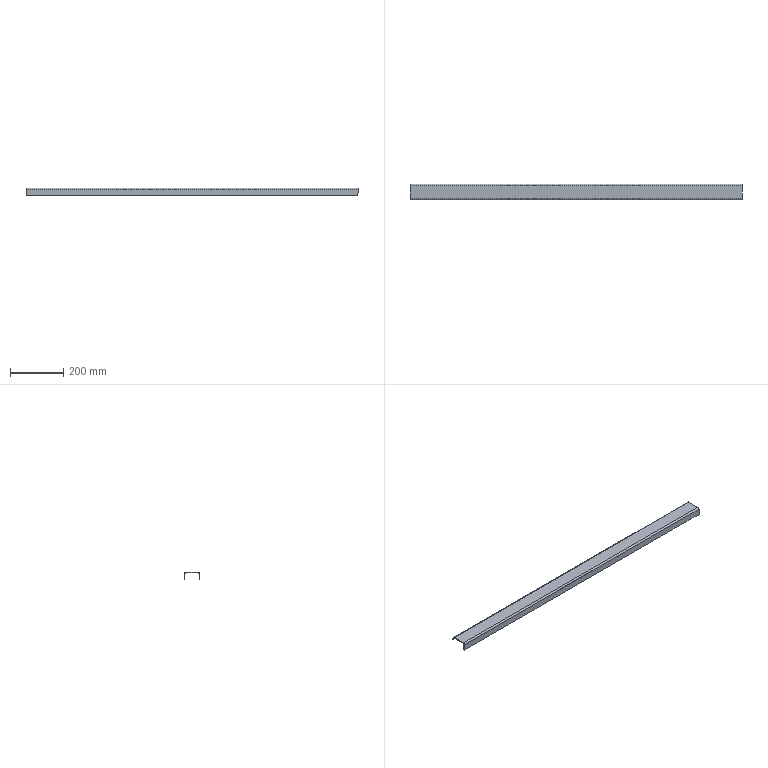Part | SolidWorks | features EdgeFlange 1, Fillet 1, FlatPattern 1, ICE 1, SMBaseFlange 1, SheetMetal 1 | 1 solid | 46 faces | box 1250 x 60 x 30 mm | volume 350614 mm3 | plane 30 | cylinder 16 | commonest cylinder face diameters 12 x14 6 x2
STEP:
#1=CARTESIAN_POINT('',(-29.,30.,-30.));
#2=VERTEX_POINT('',#1);
#3=CARTESIAN_POINT('',(29.,30.,-30.));
#4=VERTEX_POINT('',#3);
#5=CARTESIAN_POINT('',(625.,30.,-30.));
#6=DIRECTION('',(1.,0.,0.));
#7=VECTOR('',#6,1000.);
#8=LINE('',#5,#7);
#9=EDGE_CURVE('',#2,#4,#8,.T.);
#10=ORIENTED_EDGE('',*,*,#9,.T.);
#11=CARTESIAN_POINT('',(29.,27.,-30.));
#12=VERTEX_POINT('',#11);
#13=CARTESIAN_POINT('',(29.,27.,-30.));
#14=DIRECTION('',(0.,-1.,0.));
#15=VECTOR('',#14,1000.);
#16=LINE('',#13,#15);
#17=EDGE_CURVE('',#4,#12,#16,.T.);
#18=ORIENTED_EDGE('',*,*,#17,.T.);
#19=CARTESIAN_POINT('',(-29.,27.,-30.));
#20=VERTEX_POINT('',#19);
#21=CARTESIAN_POINT('',(0.,27.,-30.));
#22=DIRECTION('',(1.,0.,0.));
#23=VECTOR('',#22,1000.);
#24=LINE('',#21,#23);
#25=EDGE_CURVE('',#20,#12,#24,.T.);
#26=ORIENTED_EDGE('',*,*,#25,.F.);
#27=CARTESIAN_POINT('',(-29.,30.,-30.));
#28=DIRECTION('',(0.,1.,0.));
#29=VECTOR('',#28,1000.);
#30=LINE('',#27,#29);
#31=EDGE_CURVE('',#20,#2,#30,.T.);
#32=ORIENTED_EDGE('',*,*,#31,.T.);
#33=EDGE_LOOP('',(#10,#18,#26,#32));
#34=FACE_OUTER_BOUND('',#33,.T.);
#35=CARTESIAN_POINT('',(625.,30.,-30.));
#36=DIRECTION('',(0.,0.,-1.));
#37=DIRECTION('',(0.,1.,0.));
#38=AXIS2_PLACEMENT_3D('',#35,#36,#37);
#39=PLANE('',#38);
#40=ADVANCED_FACE('',(#34),#39,.T.);
#41=CARTESIAN_POINT('',(406.,27.,-30.));
#42=VERTEX_POINT('',#41);
#43=CARTESIAN_POINT('',(464.,27.,-30.));
#44=VERTEX_POINT('',#43);
#45=CARTESIAN_POINT('',(0.,27.,-30.));
#46=DIRECTION('',(1.,0.,0.));
#47=VECTOR('',#46,1000.);
#48=LINE('',#45,#47);
#49=EDGE_CURVE('',#42,#44,#48,.T.);
#50=ORIENTED_EDGE('',*,*,#49,.F.);
#51=CARTESIAN_POINT('',(406.,30.,-30.));
#52=VERTEX_POINT('',#51);
#53=CARTESIAN_POINT('',(406.,30.,-30.));
#54=DIRECTION('',(0.,1.,0.));
#55=VECTOR('',#54,1000.);
#56=LINE('',#53,#55);
#57=EDGE_CURVE('',#42,#52,#56,.T.);
#58=ORIENTED_EDGE('',*,*,#57,.T.);
#59=CARTESIAN_POINT('',(464.,30.,-30.));
#60=VERTEX_POINT('',#59);
#61=CARTESIAN_POINT('',(625.,30.,-30.));
#62=DIRECTION('',(1.,0.,0.));
#63=VECTOR('',#62,1000.);
#64=LINE('',#61,#63);
#65=EDGE_CURVE('',#52,#60,#64,.T.);
#66=ORIENTED_EDGE('',*,*,#65,.T.);
#67=CARTESIAN_POINT('',(464.,27.,-30.));
#68=DIRECTION('',(0.,-1.,0.));
#69=VECTOR('',#68,1000.);
#70=LINE('',#67,#69);
#71=EDGE_CURVE('',#60,#44,#70,.T.);
#72=ORIENTED_EDGE('',*,*,#71,.T.);
#73=EDGE_LOOP('',(#50,#58,#66,#72));
#74=FACE_OUTER_BOUND('',#73,.T.);
#75=CARTESIAN_POINT('',(625.,30.,-30.));
#76=DIRECTION('',(0.,0.,-1.));
#77=DIRECTION('',(0.,1.,0.));
#78=AXIS2_PLACEMENT_3D('',#75,#76,#77);
#79=PLANE('',#78);
#80=ADVANCED_FACE('',(#74),#79,.T.);
#81=CARTESIAN_POINT('',(625.,-24.,-3.));
#82=VERTEX_POINT('',#81);
#83=CARTESIAN_POINT('',(625.,24.,-3.));
#84=VERTEX_POINT('',#83);
#85=CARTESIAN_POINT('',(625.,-30.,-3.));
#86=DIRECTION('',(0.,1.,0.));
#87=VECTOR('',#86,1000.);
#88=LINE('',#85,#87);
#89=EDGE_CURVE('',#82,#84,#88,.T.);
#90=ORIENTED_EDGE('',*,*,#89,.F.);
#91=CARTESIAN_POINT('',(-625.,-24.,-3.));
#92=VERTEX_POINT('',#91);
#93=CARTESIAN_POINT('',(-625.,-24.,-3.));
#94=DIRECTION('',(1.,0.,0.));
#95=VECTOR('',#94,1000.);
#96=LINE('',#93,#95);
#97=EDGE_CURVE('',#92,#82,#96,.T.);
#98=ORIENTED_EDGE('',*,*,#97,.F.);
#99=CARTESIAN_POINT('',(-625.,24.,-3.));
#100=VERTEX_POINT('',#99);
#101=CARTESIAN_POINT('',(-625.,-30.,-3.));
#102=DIRECTION('',(0.,-1.,0.));
#103=VECTOR('',#102,1000.);
#104=LINE('',#101,#103);
#105=EDGE_CURVE('',#100,#92,#104,.T.);
#106=ORIENTED_EDGE('',*,*,#105,.F.);
#107=CARTESIAN_POINT('',(625.,24.,-3.));
#108=DIRECTION('',(-1.,0.,0.));
#109=VECTOR('',#108,1000.);
#110=LINE('',#107,#109);
#111=EDGE_CURVE('',#84,#100,#110,.T.);
#112=ORIENTED_EDGE('',*,*,#111,.F.);
#113=EDGE_LOOP('',(#90,#98,#106,#112));
#114=FACE_OUTER_BOUND('',#113,.T.);
#115=CARTESIAN_POINT('',(0.,0.,-3.));
#116=DIRECTION('',(0.,0.,-1.));
#117=DIRECTION('',(-1.,0.,0.));
#118=AXIS2_PLACEMENT_3D('',#115,#116,#117);
#119=PLANE('',#118);
#120=ADVANCED_FACE('',(#114),#119,.T.);
#121=CARTESIAN_POINT('',(-625.,-24.,0.));
#122=VERTEX_POINT('',#121);
#123=CARTESIAN_POINT('',(625.,-24.,0.));
#124=VERTEX_POINT('',#123);
#125=CARTESIAN_POINT('',(-625.,-24.,0.));
#126=DIRECTION('',(1.,0.,0.));
#127=VECTOR('',#126,1000.);
#128=LINE('',#125,#127);
#129=EDGE_CURVE('',#122,#124,#128,.T.);
#130=ORIENTED_EDGE('',*,*,#129,.T.);
#131=CARTESIAN_POINT('',(625.,24.,0.));
#132=VERTEX_POINT('',#131);
#133=CARTESIAN_POINT('',(625.,-30.,0.));
#134=DIRECTION('',(0.,1.,0.));
#135=VECTOR('',#134,1000.);
#136=LINE('',#133,#135);
#137=EDGE_CURVE('',#124,#132,#136,.T.);
#138=ORIENTED_EDGE('',*,*,#137,.T.);
#139=CARTESIAN_POINT('',(-625.,24.,0.));
#140=VERTEX_POINT('',#139);
#141=CARTESIAN_POINT('',(625.,24.,0.));
#142=DIRECTION('',(-1.,0.,0.));
#143=VECTOR('',#142,1000.);
#144=LINE('',#141,#143);
#145=EDGE_CURVE('',#132,#140,#144,.T.);
#146=ORIENTED_EDGE('',*,*,#145,.T.);
#147=CARTESIAN_POINT('',(-625.,-30.,0.));
#148=DIRECTION('',(0.,-1.,0.));
#149=VECTOR('',#148,1000.);
#150=LINE('',#147,#149);
#151=EDGE_CURVE('',#140,#122,#150,.T.);
#152=ORIENTED_EDGE('',*,*,#151,.T.);
#153=EDGE_LOOP('',(#130,#138,#146,#152));
#154=FACE_OUTER_BOUND('',#153,.T.);
#155=CARTESIAN_POINT('',(0.,0.,0.));
#156=DIRECTION('',(0.,0.,-1.));
#157=DIRECTION('',(-1.,0.,0.));
#158=AXIS2_PLACEMENT_3D('',#155,#156,#157);
#159=PLANE('',#158);
#160=ADVANCED_FACE('',(#154),#159,.F.);
#161=ORIENTED_EDGE('',*,*,#105,.T.);
#162=CARTESIAN_POINT('',(-625.,-24.,-3.));
#163=DIRECTION('',(0.,0.,1.));
#164=VECTOR('',#163,1000.);
#165=LINE('',#162,#164);
#166=EDGE_CURVE('',#92,#122,#165,.T.);
#167=ORIENTED_EDGE('',*,*,#166,.T.);
#168=ORIENTED_EDGE('',*,*,#151,.F.);
#169=CARTESIAN_POINT('',(-625.,24.,-3.));
#170=DIRECTION('',(0.,0.,1.));
#171=VECTOR('',#170,1000.);
#172=LINE('',#169,#171);
#173=EDGE_CURVE('',#100,#140,#172,.T.);
#174=ORIENTED_EDGE('',*,*,#173,.F.);
#175=EDGE_LOOP('',(#161,#167,#168,#174));
#176=FACE_OUTER_BOUND('',#175,.T.);
#177=CARTESIAN_POINT('',(-625.,-30.,-3.));
#178=DIRECTION('',(-1.,0.,0.));
#179=DIRECTION('',(0.,0.,1.));
#180=AXIS2_PLACEMENT_3D('',#177,#178,#179);
#181=PLANE('',#180);
#182=ADVANCED_FACE('',(#176),#181,.T.);
#183=CARTESIAN_POINT('',(625.,-24.,-3.));
#184=DIRECTION('',(0.,0.,1.));
#185=VECTOR('',#184,1000.);
#186=LINE('',#183,#185);
#187=EDGE_CURVE('',#82,#124,#186,.T.);
#188=ORIENTED_EDGE('',*,*,#187,.F.);
#189=ORIENTED_EDGE('',*,*,#89,.T.);
#190=CARTESIAN_POINT('',(625.,24.,-3.));
#191=DIRECTION('',(0.,0.,1.));
#192=VECTOR('',#191,1000.);
#193=LINE('',#190,#192);
#194=EDGE_CURVE('',#84,#132,#193,.T.);
#195=ORIENTED_EDGE('',*,*,#194,.T.);
#196=ORIENTED_EDGE('',*,*,#137,.F.);
#197=EDGE_LOOP('',(#188,#189,#195,#196));
#198=FACE_OUTER_BOUND('',#197,.T.);
#199=CARTESIAN_POINT('',(625.,-30.,-3.));
#200=DIRECTION('',(1.,0.,0.));
#201=DIRECTION('',(0.,0.,-1.));
#202=AXIS2_PLACEMENT_3D('',#199,#200,#201);
#203=PLANE('',#202);
#204=ADVANCED_FACE('',(#198),#203,.T.);
#205=CARTESIAN_POINT('',(-625.,27.,-6.));
#206=VERTEX_POINT('',#205);
#207=CARTESIAN_POINT('',(-625.,30.,-6.));
#208=VERTEX_POINT('',#207);
#209=CARTESIAN_POINT('',(-625.,30.,-6.));
#210=DIRECTION('',(0.,1.,0.));
#211=VECTOR('',#210,1000.);
#212=LINE('',#209,#211);
#213=EDGE_CURVE('',#206,#208,#212,.T.);
#214=ORIENTED_EDGE('',*,*,#213,.F.);
#215=CARTESIAN_POINT('',(-625.,24.,-6.));
#216=DIRECTION('',(-1.,0.,0.));
#217=DIRECTION('',(0.,0.,-1.));
#218=AXIS2_PLACEMENT_3D('',#215,#216,#217);
#219=CIRCLE('',#218,3.);
#220=EDGE_CURVE('',#100,#206,#219,.T.);
#221=ORIENTED_EDGE('',*,*,#220,.F.);
#222=ORIENTED_EDGE('',*,*,#173,.T.);
#223=CARTESIAN_POINT('',(-625.,24.,-6.));
#224=DIRECTION('',(-1.,0.,0.));
#225=DIRECTION('',(0.,0.,-1.));
#226=AXIS2_PLACEMENT_3D('',#223,#224,#225);
#227=CIRCLE('',#226,6.);
#228=EDGE_CURVE('',#140,#208,#227,.T.);
#229=ORIENTED_EDGE('',*,*,#228,.T.);
#230=EDGE_LOOP('',(#214,#221,#222,#229));
#231=FACE_OUTER_BOUND('',#230,.T.);
#232=CARTESIAN_POINT('',(-625.,24.,-6.));
#233=DIRECTION('',(-1.,0.,0.));
#234=DIRECTION('',(0.,0.,1.));
#235=AXIS2_PLACEMENT_3D('',#232,#233,#234);
#236=PLANE('',#235);
#237=ADVANCED_FACE('',(#231),#236,.T.);
#238=CARTESIAN_POINT('',(625.,27.,-6.));
#239=VERTEX_POINT('',#238);
#240=CARTESIAN_POINT('',(625.,24.,-6.));
#241=DIRECTION('',(1.,0.,0.));
#242=DIRECTION('',(0.,0.,-1.));
#243=AXIS2_PLACEMENT_3D('',#240,#241,#242);
#244=CIRCLE('',#243,3.);
#245=EDGE_CURVE('',#239,#84,#244,.T.);
#246=ORIENTED_EDGE('',*,*,#245,.F.);
#247=CARTESIAN_POINT('',(625.,30.,-6.));
#248=VERTEX_POINT('',#247);
#249=CARTESIAN_POINT('',(625.,27.,-6.));
#250=DIRECTION('',(0.,1.,0.));
#251=VECTOR('',#250,1000.);
#252=LINE('',#249,#251);
#253=EDGE_CURVE('',#239,#248,#252,.T.);
#254=ORIENTED_EDGE('',*,*,#253,.T.);
#255=CARTESIAN_POINT('',(625.,24.,-6.));
#256=DIRECTION('',(1.,0.,0.));
#257=DIRECTION('',(0.,0.,-1.));
#258=AXIS2_PLACEMENT_3D('',#255,#256,#257);
#259=CIRCLE('',#258,6.);
#260=EDGE_CURVE('',#248,#132,#259,.T.);
#261=ORIENTED_EDGE('',*,*,#260,.T.);
#262=ORIENTED_EDGE('',*,*,#194,.F.);
#263=EDGE_LOOP('',(#246,#254,#261,#262));
#264=FACE_OUTER_BOUND('',#263,.T.);
#265=CARTESIAN_POINT('',(625.,24.,-6.));
#266=DIRECTION('',(-1.,0.,0.));
#267=DIRECTION('',(0.,0.,1.));
#268=AXIS2_PLACEMENT_3D('',#265,#266,#267);
#269=PLANE('',#268);
#270=ADVANCED_FACE('',(#264),#269,.F.);
#271=ORIENTED_EDGE('',*,*,#145,.F.);
#272=ORIENTED_EDGE('',*,*,#260,.F.);
#273=CARTESIAN_POINT('',(0.,30.,-6.));
#274=DIRECTION('',(1.,0.,0.));
#275=VECTOR('',#274,1000.);
#276=LINE('',#273,#275);
#277=EDGE_CURVE('',#208,#248,#276,.T.);
#278=ORIENTED_EDGE('',*,*,#277,.F.);
#279=ORIENTED_EDGE('',*,*,#228,.F.);
#280=EDGE_LOOP('',(#271,#272,#278,#279));
#281=FACE_OUTER_BOUND('',#280,.T.);
#282=CARTESIAN_POINT('',(625.,24.,-6.));
#283=DIRECTION('',(1.,0.,0.));
#284=DIRECTION('',(0.,1.,0.));
#285=AXIS2_PLACEMENT_3D('',#282,#283,#284);
#286=CYLINDRICAL_SURFACE('',#285,6.);
#287=ADVANCED_FACE('',(#281),#286,.T.);
#288=ORIENTED_EDGE('',*,*,#111,.T.);
#289=ORIENTED_EDGE('',*,*,#220,.T.);
#290=CARTESIAN_POINT('',(-625.,27.,-6.));
#291=DIRECTION('',(1.,0.,0.));
#292=VECTOR('',#291,1000.);
#293=LINE('',#290,#292);
#294=EDGE_CURVE('',#206,#239,#293,.T.);
#295=ORIENTED_EDGE('',*,*,#294,.T.);
#296=ORIENTED_EDGE('',*,*,#245,.T.);
#297=EDGE_LOOP('',(#288,#289,#295,#296));
#298=FACE_OUTER_BOUND('',#297,.T.);
#299=CARTESIAN_POINT('',(625.,24.,-6.));
#300=DIRECTION('',(1.,0.,0.));
#301=DIRECTION('',(0.,1.,0.));
#302=AXIS2_PLACEMENT_3D('',#299,#300,#301);
#303=CYLINDRICAL_SURFACE('',#302,3.);
#304=ADVANCED_FACE('',(#298),#303,.F.);
#305=CARTESIAN_POINT('',(625.,27.,-10.));
#306=VERTEX_POINT('',#305);
#307=CARTESIAN_POINT('',(625.,30.,-10.));
#308=VERTEX_POINT('',#307);
#309=CARTESIAN_POINT('',(625.,20.,-10.));
#310=DIRECTION('',(0.,1.,0.));
#311=VECTOR('',#310,1000.);
#312=LINE('',#309,#311);
#313=EDGE_CURVE('',#306,#308,#312,.T.);
#314=ORIENTED_EDGE('',*,*,#313,.T.);
#315=CARTESIAN_POINT('',(625.,30.,-3.));
#316=DIRECTION('',(0.,0.,1.));
#317=VECTOR('',#316,1000.);
#318=LINE('',#315,#317);
#319=EDGE_CURVE('',#308,#248,#318,.T.);
#320=ORIENTED_EDGE('',*,*,#319,.T.);
#321=ORIENTED_EDGE('',*,*,#253,.F.);
#322=CARTESIAN_POINT('',(625.,27.,0.));
#323=DIRECTION('',(0.,0.,1.));
#324=VECTOR('',#323,1000.);
#325=LINE('',#322,#324);
#326=EDGE_CURVE('',#306,#239,#325,.T.);
#327=ORIENTED_EDGE('',*,*,#326,.F.);
#328=EDGE_LOOP('',(#314,#320,#321,#327));
#329=FACE_OUTER_BOUND('',#328,.T.);
#330=CARTESIAN_POINT('',(625.,30.,-3.));
#331=DIRECTION('',(1.,0.,0.));
#332=DIRECTION('',(0.,0.,-1.));
#333=AXIS2_PLACEMENT_3D('',#330,#331,#332);
#334=PLANE('',#333);
#335=ADVANCED_FACE('',(#329),#334,.T.);
#336=CARTESIAN_POINT('',(-625.,27.,-10.));
#337=VERTEX_POINT('',#336);
#338=CARTESIAN_POINT('',(-625.,30.,-10.));
#339=VERTEX_POINT('',#338);
#340=CARTESIAN_POINT('',(-625.,20.,-10.));
#341=DIRECTION('',(0.,1.,0.));
#342=VECTOR('',#341,1000.);
#343=LINE('',#340,#342);
#344=EDGE_CURVE('',#337,#339,#343,.T.);
#345=ORIENTED_EDGE('',*,*,#344,.F.);
#346=CARTESIAN_POINT('',(-625.,27.,0.));
#347=DIRECTION('',(0.,0.,-1.));
#348=VECTOR('',#347,1000.);
#349=LINE('',#346,#348);
#350=EDGE_CURVE('',#206,#337,#349,.T.);
#351=ORIENTED_EDGE('',*,*,#350,.F.);
#352=ORIENTED_EDGE('',*,*,#213,.T.);
#353=CARTESIAN_POINT('',(-625.,30.,-30.));
#354=DIRECTION('',(0.,0.,-1.));
#355=VECTOR('',#354,1000.);
#356=LINE('',#353,#355);
#357=EDGE_CURVE('',#208,#339,#356,.T.);
#358=ORIENTED_EDGE('',*,*,#357,.T.);
#359=EDGE_LOOP('',(#345,#351,#352,#358));
#360=FACE_OUTER_BOUND('',#359,.T.);
#361=CARTESIAN_POINT('',(-625.,30.,-30.));
#362=DIRECTION('',(-1.,0.,0.));
#363=DIRECTION('',(0.,0.,1.));
#364=AXIS2_PLACEMENT_3D('',#361,#362,#363);
#365=PLANE('',#364);
#366=ADVANCED_FACE('',(#360),#365,.T.);
#367=CARTESIAN_POINT('',(-464.,30.,-30.));
#368=VERTEX_POINT('',#367);
#369=CARTESIAN_POINT('',(-406.,30.,-30.));
#370=VERTEX_POINT('',#369);
#371=CARTESIAN_POINT('',(625.,30.,-30.));
#372=DIRECTION('',(1.,0.,0.));
#373=VECTOR('',#372,1000.);
#374=LINE('',#371,#373);
#375=EDGE_CURVE('',#368,#370,#374,.T.);
#376=ORIENTED_EDGE('',*,*,#375,.F.);
#377=CARTESIAN_POINT('',(-470.,30.,-24.));
#378=VERTEX_POINT('',#377);
#379=CARTESIAN_POINT('',(-464.,30.,-24.));
#380=DIRECTION('',(0.,1.,0.));
#381=DIRECTION('',(0.,0.,1.));
#382=AXIS2_PLACEMENT_3D('',#379,#380,#381);
#383=CIRCLE('',#382,6.);
#384=EDGE_CURVE('',#368,#378,#383,.T.);
#385=ORIENTED_EDGE('',*,*,#384,.T.);
#386=CARTESIAN_POINT('',(-470.,30.,-16.));
#387=VERTEX_POINT('',#386);
#388=CARTESIAN_POINT('',(-470.,30.,-30.));
#389=DIRECTION('',(0.,0.,-1.));
#390=VECTOR('',#389,1000.);
#391=LINE('',#388,#390);
#392=EDGE_CURVE('',#387,#378,#391,.T.);
#393=ORIENTED_EDGE('',*,*,#392,.F.);
#394=CARTESIAN_POINT('',(-476.,30.,-10.));
#395=VERTEX_POINT('',#394);
#396=CARTESIAN_POINT('',(-476.,30.,-16.));
#397=DIRECTION('',(0.,-1.,0.));
#398=DIRECTION('',(0.,0.,1.));
#399=AXIS2_PLACEMENT_3D('',#396,#397,#398);
#400=CIRCLE('',#399,6.);
#401=EDGE_CURVE('',#387,#395,#400,.T.);
#402=ORIENTED_EDGE('',*,*,#401,.T.);
#403=CARTESIAN_POINT('',(-470.,30.,-10.));
#404=DIRECTION('',(1.,0.,0.));
#405=VECTOR('',#404,1000.);
#406=LINE('',#403,#405);
#407=EDGE_CURVE('',#339,#395,#406,.T.);
#408=ORIENTED_EDGE('',*,*,#407,.F.);
#409=ORIENTED_EDGE('',*,*,#357,.F.);
#410=ORIENTED_EDGE('',*,*,#277,.T.);
#411=ORIENTED_EDGE('',*,*,#319,.F.);
#412=CARTESIAN_POINT('',(476.,30.,-10.));
#413=VERTEX_POINT('',#412);
#414=CARTESIAN_POINT('',(470.,30.,-10.));
#415=DIRECTION('',(1.,0.,0.));
#416=VECTOR('',#415,1000.);
#417=LINE('',#414,#416);
#418=EDGE_CURVE('',#413,#308,#417,.T.);
#419=ORIENTED_EDGE('',*,*,#418,.F.);
#420=CARTESIAN_POINT('',(470.,30.,-16.));
#421=VERTEX_POINT('',#420);
#422=CARTESIAN_POINT('',(476.,30.,-16.));
#423=DIRECTION('',(0.,-1.,0.));
#424=DIRECTION('',(0.,0.,1.));
#425=AXIS2_PLACEMENT_3D('',#422,#423,#424);
#426=CIRCLE('',#425,6.);
#427=EDGE_CURVE('',#413,#421,#426,.T.);
#428=ORIENTED_EDGE('',*,*,#427,.T.);
#429=CARTESIAN_POINT('',(470.,30.,-24.));
#430=VERTEX_POINT('',#429);
#431=CARTESIAN_POINT('',(470.,30.,-30.));
#432=DIRECTION('',(0.,0.,1.));
#433=VECTOR('',#432,1000.);
#434=LINE('',#431,#433);
#435=EDGE_CURVE('',#430,#421,#434,.T.);
#436=ORIENTED_EDGE('',*,*,#435,.F.);
#437=CARTESIAN_POINT('',(464.,30.,-24.));
#438=DIRECTION('',(0.,1.,0.));
#439=DIRECTION('',(0.,0.,1.));
#440=AXIS2_PLACEMENT_3D('',#437,#438,#439);
#441=CIRCLE('',#440,6.);
#442=EDGE_CURVE('',#430,#60,#441,.T.);
#443=ORIENTED_EDGE('',*,*,#442,.T.);
#444=ORIENTED_EDGE('',*,*,#65,.F.);
#445=CARTESIAN_POINT('',(400.,30.,-24.));
#446=VERTEX_POINT('',#445);
#447=CARTESIAN_POINT('',(406.,30.,-24.));
#448=DIRECTION('',(0.,1.,0.));
#449=DIRECTION('',(0.,0.,1.));
#450=AXIS2_PLACEMENT_3D('',#447,#448,#449);
#451=CIRCLE('',#450,6.);
#452=EDGE_CURVE('',#52,#446,#451,.T.);
#453=ORIENTED_EDGE('',*,*,#452,.T.);
#454=CARTESIAN_POINT('',(400.,30.,-16.));
#455=VERTEX_POINT('',#454);
#456=CARTESIAN_POINT('',(400.,30.,-30.));
#457=DIRECTION('',(0.,0.,-1.));
#458=VECTOR('',#457,1000.);
#459=LINE('',#456,#458);
#460=EDGE_CURVE('',#455,#446,#459,.T.);
#461=ORIENTED_EDGE('',*,*,#460,.F.);
#462=CARTESIAN_POINT('',(394.,30.,-10.));
#463=VERTEX_POINT('',#462);
#464=CARTESIAN_POINT('',(394.,30.,-16.));
#465=DIRECTION('',(0.,-1.,0.));
#466=DIRECTION('',(0.,0.,1.));
#467=AXIS2_PLACEMENT_3D('',#464,#465,#466);
#468=CIRCLE('',#467,6.);
#469=EDGE_CURVE('',#455,#463,#468,.T.);
#470=ORIENTED_EDGE('',*,*,#469,.T.);
#471=CARTESIAN_POINT('',(41.,30.,-10.));
#472=VERTEX_POINT('',#471);
#473=CARTESIAN_POINT('',(400.,30.,-10.));
#474=DIRECTION('',(1.,0.,0.));
#475=VECTOR('',#474,1000.);
#476=LINE('',#473,#475);
#477=EDGE_CURVE('',#472,#463,#476,.T.);
#478=ORIENTED_EDGE('',*,*,#477,.F.);
#479=CARTESIAN_POINT('',(35.,30.,-16.));
#480=VERTEX_POINT('',#479);
#481=CARTESIAN_POINT('',(41.,30.,-16.));
#482=DIRECTION('',(0.,-1.,0.));
#483=DIRECTION('',(0.,0.,1.));
#484=AXIS2_PLACEMENT_3D('',#481,#482,#483);
#485=CIRCLE('',#484,6.);
#486=EDGE_CURVE('',#472,#480,#485,.T.);
#487=ORIENTED_EDGE('',*,*,#486,.T.);
#488=CARTESIAN_POINT('',(35.,30.,-24.));
#489=VERTEX_POINT('',#488);
#490=CARTESIAN_POINT('',(35.,30.,-30.));
#491=DIRECTION('',(0.,0.,1.));
#492=VECTOR('',#491,1000.);
#493=LINE('',#490,#492);
#494=EDGE_CURVE('',#489,#480,#493,.T.);
#495=ORIENTED_EDGE('',*,*,#494,.F.);
#496=CARTESIAN_POINT('',(29.,30.,-24.));
#497=DIRECTION('',(0.,1.,0.));
#498=DIRECTION('',(0.,0.,1.));
#499=AXIS2_PLACEMENT_3D('',#496,#497,#498);
#500=CIRCLE('',#499,6.);
#501=EDGE_CURVE('',#489,#4,#500,.T.);
#502=ORIENTED_EDGE('',*,*,#501,.T.);
#503=ORIENTED_EDGE('',*,*,#9,.F.);
#504=CARTESIAN_POINT('',(-35.,30.,-24.));
#505=VERTEX_POINT('',#504);
#506=CARTESIAN_POINT('',(-29.,30.,-24.));
#507=DIRECTION('',(0.,1.,0.));
#508=DIRECTION('',(0.,0.,1.));
#509=AXIS2_PLACEMENT_3D('',#506,#507,#508);
#510=CIRCLE('',#509,6.);
#511=EDGE_CURVE('',#2,#505,#510,.T.);
#512=ORIENTED_EDGE('',*,*,#511,.T.);
#513=CARTESIAN_POINT('',(-35.,30.,-16.));
#514=VERTEX_POINT('',#513);
#515=CARTESIAN_POINT('',(-35.,30.,-30.));
#516=DIRECTION('',(0.,0.,-1.));
#517=VECTOR('',#516,1000.);
#518=LINE('',#515,#517);
#519=EDGE_CURVE('',#514,#505,#518,.T.);
#520=ORIENTED_EDGE('',*,*,#519,.F.);
#521=CARTESIAN_POINT('',(-41.,30.,-10.));
#522=VERTEX_POINT('',#521);
#523=CARTESIAN_POINT('',(-41.,30.,-16.));
#524=DIRECTION('',(0.,-1.,0.));
#525=DIRECTION('',(0.,0.,1.));
#526=AXIS2_PLACEMENT_3D('',#523,#524,#525);
#527=CIRCLE('',#526,6.);
#528=EDGE_CURVE('',#514,#522,#527,.T.);
#529=ORIENTED_EDGE('',*,*,#528,.T.);
#530=CARTESIAN_POINT('',(-394.,30.,-10.));
#531=VERTEX_POINT('',#530);
#532=CARTESIAN_POINT('',(-35.,30.,-10.));
#533=DIRECTION('',(1.,0.,0.));
#534=VECTOR('',#533,1000.);
#535=LINE('',#532,#534);
#536=EDGE_CURVE('',#531,#522,#535,.T.);
#537=ORIENTED_EDGE('',*,*,#536,.F.);
#538=CARTESIAN_POINT('',(-400.,30.,-16.));
#539=VERTEX_POINT('',#538);
#540=CARTESIAN_POINT('',(-394.,30.,-16.));
#541=DIRECTION('',(0.,-1.,0.));
#542=DIRECTION('',(0.,0.,1.));
#543=AXIS2_PLACEMENT_3D('',#540,#541,#542);
#544=CIRCLE('',#543,6.);
#545=EDGE_CURVE('',#531,#539,#544,.T.);
#546=ORIENTED_EDGE('',*,*,#545,.T.);
#547=CARTESIAN_POINT('',(-400.,30.,-24.));
#548=VERTEX_POINT('',#547);
#549=CARTESIAN_POINT('',(-400.,30.,-30.));
#550=DIRECTION('',(0.,0.,1.));
#551=VECTOR('',#550,1000.);
#552=LINE('',#549,#551);
#553=EDGE_CURVE('',#548,#539,#552,.T.);
#554=ORIENTED_EDGE('',*,*,#553,.F.);
#555=CARTESIAN_POINT('',(-406.,30.,-24.));
#556=DIRECTION('',(0.,1.,0.));
#557=DIRECTION('',(0.,0.,1.));
#558=AXIS2_PLACEMENT_3D('',#555,#556,#557);
#559=CIRCLE('',#558,6.);
#560=EDGE_CURVE('',#548,#370,#559,.T.);
#561=ORIENTED_EDGE('',*,*,#560,.T.);
#562=EDGE_LOOP('',(#376,#385,#393,#402,#408,#409,#410,#411,#419,#428,#436,#443,#444,#453,#461,#470,#478,#487,#495,#502,#503,#512,#520,#529,#537,#546,#554,#561));
#563=FACE_OUTER_BOUND('',#562,.T.);
#564=CARTESIAN_POINT('',(0.,30.,0.));
#565=DIRECTION('',(0.,1.,0.));
#566=DIRECTION('',(0.,0.,1.));
#567=AXIS2_PLACEMENT_3D('',#564,#565,#566);
#568=PLANE('',#567);
#569=ADVANCED_FACE('',(#563),#568,.T.);
#570=CARTESIAN_POINT('',(-470.,27.,-16.));
#571=VERTEX_POINT('',#570);
#572=CARTESIAN_POINT('',(-470.,27.,-24.));
#573=VERTEX_POINT('',#572);
#574=CARTESIAN_POINT('',(-470.,27.,0.));
#575=DIRECTION('',(0.,0.,-1.));
#576=VECTOR('',#575,1000.);
#577=LINE('',#574,#576);
#578=EDGE_CURVE('',#571,#573,#577,.T.);
#579=ORIENTED_EDGE('',*,*,#578,.T.);
#580=CARTESIAN_POINT('',(-464.,27.,-30.));
#581=VERTEX_POINT('',#580);
#582=CARTESIAN_POINT('',(-464.,27.,-24.));
#583=DIRECTION('',(0.,-1.,0.));
#584=DIRECTION('',(0.,0.,1.));
#585=AXIS2_PLACEMENT_3D('',#582,#583,#584);
#586=CIRCLE('',#585,6.);
#587=EDGE_CURVE('',#573,#581,#586,.T.);
#588=ORIENTED_EDGE('',*,*,#587,.T.);
#589=CARTESIAN_POINT('',(-406.,27.,-30.));
#590=VERTEX_POINT('',#589);
#591=CARTESIAN_POINT('',(0.,27.,-30.));
#592=DIRECTION('',(1.,0.,0.));
#593=VECTOR('',#592,1000.);
#594=LINE('',#591,#593);
#595=EDGE_CURVE('',#581,#590,#594,.T.);
#596=ORIENTED_EDGE('',*,*,#595,.T.);
#597=CARTESIAN_POINT('',(-400.,27.,-24.));
#598=VERTEX_POINT('',#597);
#599=CARTESIAN_POINT('',(-406.,27.,-24.));
#600=DIRECTION('',(0.,-1.,0.));
#601=DIRECTION('',(0.,0.,1.));
#602=AXIS2_PLACEMENT_3D('',#599,#600,#601);
#603=CIRCLE('',#602,6.);
#604=EDGE_CURVE('',#590,#598,#603,.T.);
#605=ORIENTED_EDGE('',*,*,#604,.T.);
#606=CARTESIAN_POINT('',(-400.,27.,-16.));
#607=VERTEX_POINT('',#606);
#608=CARTESIAN_POINT('',(-400.,27.,0.));
#609=DIRECTION('',(0.,0.,1.));
#610=VECTOR('',#609,1000.);
#611=LINE('',#608,#610);
#612=EDGE_CURVE('',#598,#607,#611,.T.);
#613=ORIENTED_EDGE('',*,*,#612,.T.);
#614=CARTESIAN_POINT('',(-394.,27.,-10.));
#615=VERTEX_POINT('',#614);
#616=CARTESIAN_POINT('',(-394.,27.,-16.));
#617=DIRECTION('',(0.,1.,0.));
#618=DIRECTION('',(0.,0.,1.));
#619=AXIS2_PLACEMENT_3D('',#616,#617,#618);
#620=CIRCLE('',#619,6.);
#621=EDGE_CURVE('',#607,#615,#620,.T.);
#622=ORIENTED_EDGE('',*,*,#621,.T.);
#623=CARTESIAN_POINT('',(-41.,27.,-10.));
#624=VERTEX_POINT('',#623);
#625=CARTESIAN_POINT('',(0.,27.,-10.));
#626=DIRECTION('',(1.,0.,0.));
#627=VECTOR('',#626,1000.);
#628=LINE('',#625,#627);
#629=EDGE_CURVE('',#615,#624,#628,.T.);
#630=ORIENTED_EDGE('',*,*,#629,.T.);
#631=CARTESIAN_POINT('',(-35.,27.,-16.));
#632=VERTEX_POINT('',#631);
#633=CARTESIAN_POINT('',(-41.,27.,-16.));
#634=DIRECTION('',(0.,1.,0.));
#635=DIRECTION('',(0.,0.,1.));
#636=AXIS2_PLACEMENT_3D('',#633,#634,#635);
#637=CIRCLE('',#636,6.);
#638=EDGE_CURVE('',#624,#632,#637,.T.);
#639=ORIENTED_EDGE('',*,*,#638,.T.);
#640=CARTESIAN_POINT('',(-35.,27.,-24.));
#641=VERTEX_POINT('',#640);
#642=CARTESIAN_POINT('',(-35.,27.,0.));
#643=DIRECTION('',(0.,0.,-1.));
#644=VECTOR('',#643,1000.);
#645=LINE('',#642,#644);
#646=EDGE_CURVE('',#632,#641,#645,.T.);
#647=ORIENTED_EDGE('',*,*,#646,.T.);
#648=CARTESIAN_POINT('',(-29.,27.,-24.));
#649=DIRECTION('',(0.,-1.,0.));
#650=DIRECTION('',(0.,0.,1.));
#651=AXIS2_PLACEMENT_3D('',#648,#649,#650);
#652=CIRCLE('',#651,6.);
#653=EDGE_CURVE('',#641,#20,#652,.T.);
#654=ORIENTED_EDGE('',*,*,#653,.T.);
#655=ORIENTED_EDGE('',*,*,#25,.T.);
#656=CARTESIAN_POINT('',(35.,27.,-24.));
#657=VERTEX_POINT('',#656);
#658=CARTESIAN_POINT('',(29.,27.,-24.));
#659=DIRECTION('',(0.,-1.,0.));
#660=DIRECTION('',(0.,0.,1.));
#661=AXIS2_PLACEMENT_3D('',#658,#659,#660);
#662=CIRCLE('',#661,6.);
#663=EDGE_CURVE('',#12,#657,#662,.T.);
#664=ORIENTED_EDGE('',*,*,#663,.T.);
#665=CARTESIAN_POINT('',(35.,27.,-16.));
#666=VERTEX_POINT('',#665);
#667=CARTESIAN_POINT('',(35.,27.,0.));
#668=DIRECTION('',(0.,0.,1.));
#669=VECTOR('',#668,1000.);
#670=LINE('',#667,#669);
#671=EDGE_CURVE('',#657,#666,#670,.T.);
#672=ORIENTED_EDGE('',*,*,#671,.T.);
#673=CARTESIAN_POINT('',(41.,27.,-10.));
#674=VERTEX_POINT('',#673);
#675=CARTESIAN_POINT('',(41.,27.,-16.));
#676=DIRECTION('',(0.,1.,0.));
#677=DIRECTION('',(0.,0.,1.));
#678=AXIS2_PLACEMENT_3D('',#675,#676,#677);
#679=CIRCLE('',#678,6.);
#680=EDGE_CURVE('',#666,#674,#679,.T.);
#681=ORIENTED_EDGE('',*,*,#680,.T.);
#682=CARTESIAN_POINT('',(394.,27.,-10.));
#683=VERTEX_POINT('',#682);
#684=CARTESIAN_POINT('',(0.,27.,-10.));
#685=DIRECTION('',(1.,0.,0.));
#686=VECTOR('',#685,1000.);
#687=LINE('',#684,#686);
#688=EDGE_CURVE('',#674,#683,#687,.T.);
#689=ORIENTED_EDGE('',*,*,#688,.T.);
#690=CARTESIAN_POINT('',(400.,27.,-16.));
#691=VERTEX_POINT('',#690);
#692=CARTESIAN_POINT('',(394.,27.,-16.));
#693=DIRECTION('',(0.,1.,0.));
#694=DIRECTION('',(0.,0.,1.));
#695=AXIS2_PLACEMENT_3D('',#692,#693,#694);
#696=CIRCLE('',#695,6.);
#697=EDGE_CURVE('',#683,#691,#696,.T.);
#698=ORIENTED_EDGE('',*,*,#697,.T.);
#699=CARTESIAN_POINT('',(400.,27.,-24.));
#700=VERTEX_POINT('',#699);
#701=CARTESIAN_POINT('',(400.,27.,0.));
#702=DIRECTION('',(0.,0.,-1.));
#703=VECTOR('',#702,1000.);
#704=LINE('',#701,#703);
#705=EDGE_CURVE('',#691,#700,#704,.T.);
#706=ORIENTED_EDGE('',*,*,#705,.T.);
#707=CARTESIAN_POINT('',(406.,27.,-24.));
#708=DIRECTION('',(0.,-1.,0.));
#709=DIRECTION('',(0.,0.,1.));
#710=AXIS2_PLACEMENT_3D('',#707,#708,#709);
#711=CIRCLE('',#710,6.);
#712=EDGE_CURVE('',#700,#42,#711,.T.);
#713=ORIENTED_EDGE('',*,*,#712,.T.);
#714=ORIENTED_EDGE('',*,*,#49,.T.);
#715=CARTESIAN_POINT('',(470.,27.,-24.));
#716=VERTEX_POINT('',#715);
#717=CARTESIAN_POINT('',(464.,27.,-24.));
#718=DIRECTION('',(0.,-1.,0.));
#719=DIRECTION('',(0.,0.,1.));
#720=AXIS2_PLACEMENT_3D('',#717,#718,#719);
#721=CIRCLE('',#720,6.);
#722=EDGE_CURVE('',#44,#716,#721,.T.);
#723=ORIENTED_EDGE('',*,*,#722,.T.);
#724=CARTESIAN_POINT('',(470.,27.,-16.));
#725=VERTEX_POINT('',#724);
#726=CARTESIAN_POINT('',(470.,27.,0.));
#727=DIRECTION('',(0.,0.,1.));
#728=VECTOR('',#727,1000.);
#729=LINE('',#726,#728);
#730=EDGE_CURVE('',#716,#725,#729,.T.);
#731=ORIENTED_EDGE('',*,*,#730,.T.);
#732=CARTESIAN_POINT('',(476.,27.,-10.));
#733=VERTEX_POINT('',#732);
#734=CARTESIAN_POINT('',(476.,27.,-16.));
#735=DIRECTION('',(0.,1.,0.));
#736=DIRECTION('',(0.,0.,1.));
#737=AXIS2_PLACEMENT_3D('',#734,#735,#736);
#738=CIRCLE('',#737,6.);
#739=EDGE_CURVE('',#725,#733,#738,.T.);
#740=ORIENTED_EDGE('',*,*,#739,.T.);
#741=CARTESIAN_POINT('',(0.,27.,-10.));
#742=DIRECTION('',(1.,0.,0.));
#743=VECTOR('',#742,1000.);
#744=LINE('',#741,#743);
#745=EDGE_CURVE('',#733,#306,#744,.T.);
#746=ORIENTED_EDGE('',*,*,#745,.T.);
#747=ORIENTED_EDGE('',*,*,#326,.T.);
#748=ORIENTED_EDGE('',*,*,#294,.F.);
#749=ORIENTED_EDGE('',*,*,#350,.T.);
#750=CARTESIAN_POINT('',(-476.,27.,-10.));
#751=VERTEX_POINT('',#750);
#752=CARTESIAN_POINT('',(0.,27.,-10.));
#753=DIRECTION('',(1.,0.,0.));
#754=VECTOR('',#753,1000.);
#755=LINE('',#752,#754);
#756=EDGE_CURVE('',#337,#751,#755,.T.);
#757=ORIENTED_EDGE('',*,*,#756,.T.);
#758=CARTESIAN_POINT('',(-476.,27.,-16.));
#759=DIRECTION('',(0.,1.,0.));
#760=DIRECTION('',(0.,0.,1.));
#761=AXIS2_PLACEMENT_3D('',#758,#759,#760);
#762=CIRCLE('',#761,6.);
#763=EDGE_CURVE('',#751,#571,#762,.T.);
#764=ORIENTED_EDGE('',*,*,#763,.T.);
#765=EDGE_LOOP('',(#579,#588,#596,#605,#613,#622,#630,#639,#647,#654,#655,#664,#672,#681,#689,#698,#706,#713,#714,#723,#731,#740,#746,#747,#748,#749,#757,#764));
#766=FACE_OUTER_BOUND('',#765,.T.);
#767=CARTESIAN_POINT('',(0.,27.,0.));
#768=DIRECTION('',(0.,1.,0.));
#769=DIRECTION('',(0.,0.,1.));
#770=AXIS2_PLACEMENT_3D('',#767,#768,#769);
#771=PLANE('',#770);
#772=ADVANCED_FACE('',(#766),#771,.F.);
#773=ORIENTED_EDGE('',*,*,#595,.F.);
#774=CARTESIAN_POINT('',(-464.,30.,-30.));
#775=DIRECTION('',(0.,1.,0.));
#776=VECTOR('',#775,1000.);
#777=LINE('',#774,#776);
#778=EDGE_CURVE('',#581,#368,#777,.T.);
#779=ORIENTED_EDGE('',*,*,#778,.T.);
#780=ORIENTED_EDGE('',*,*,#375,.T.);
#781=CARTESIAN_POINT('',(-406.,27.,-30.));
#782=DIRECTION('',(0.,-1.,0.));
#783=VECTOR('',#782,1000.);
#784=LINE('',#781,#783);
#785=EDGE_CURVE('',#370,#590,#784,.T.);
#786=ORIENTED_EDGE('',*,*,#785,.T.);
#787=EDGE_LOOP('',(#773,#779,#780,#786));
#788=FACE_OUTER_BOUND('',#787,.T.);
#789=CARTESIAN_POINT('',(625.,30.,-30.));
#790=DIRECTION('',(0.,0.,-1.));
#791=DIRECTION('',(0.,1.,0.));
#792=AXIS2_PLACEMENT_3D('',#789,#790,#791);
#793=PLANE('',#792);
#794=ADVANCED_FACE('',(#788),#793,.T.);
#795=CARTESIAN_POINT('',(625.,-27.,-6.));
#796=VERTEX_POINT('',#795);
#797=CARTESIAN_POINT('',(625.,-30.,-6.));
#798=VERTEX_POINT('',#797);
#799=CARTESIAN_POINT('',(625.,-30.,-6.));
#800=DIRECTION('',(0.,-1.,0.));
#801=VECTOR('',#800,1000.);
#802=LINE('',#799,#801);
#803=EDGE_CURVE('',#796,#798,#802,.T.);
#804=ORIENTED_EDGE('',*,*,#803,.F.);
#805=CARTESIAN_POINT('',(625.,-24.,-6.));
#806=DIRECTION('',(1.,0.,0.));
#807=DIRECTION('',(0.,0.,1.));
#808=AXIS2_PLACEMENT_3D('',#805,#806,#807);
#809=CIRCLE('',#808,3.);
#810=EDGE_CURVE('',#82,#796,#809,.T.);
#811=ORIENTED_EDGE('',*,*,#810,.F.);
#812=ORIENTED_EDGE('',*,*,#187,.T.);
#813=CARTESIAN_POINT('',(625.,-24.,-6.));
#814=DIRECTION('',(1.,0.,0.));
#815=DIRECTION('',(0.,0.,1.));
#816=AXIS2_PLACEMENT_3D('',#813,#814,#815);
#817=CIRCLE('',#816,6.);
#818=EDGE_CURVE('',#124,#798,#817,.T.);
#819=ORIENTED_EDGE('',*,*,#818,.T.);
#820=EDGE_LOOP('',(#804,#811,#812,#819));
#821=FACE_OUTER_BOUND('',#820,.T.);
#822=CARTESIAN_POINT('',(625.,-24.,-6.));
#823=DIRECTION('',(1.,0.,0.));
#824=DIRECTION('',(0.,0.,-1.));
#825=AXIS2_PLACEMENT_3D('',#822,#823,#824);
#826=PLANE('',#825);
#827=ADVANCED_FACE('',(#821),#826,.T.);
#828=CARTESIAN_POINT('',(-625.,-27.,-6.));
#829=VERTEX_POINT('',#828);
#830=CARTESIAN_POINT('',(-625.,-24.,-6.));
#831=DIRECTION('',(-1.,0.,0.));
#832=DIRECTION('',(0.,0.,1.));
#833=AXIS2_PLACEMENT_3D('',#830,#831,#832);
#834=CIRCLE('',#833,3.);
#835=EDGE_CURVE('',#829,#92,#834,.T.);
#836=ORIENTED_EDGE('',*,*,#835,.F.);
#837=CARTESIAN_POINT('',(-625.,-30.,-6.));
#838=VERTEX_POINT('',#837);
#839=CARTESIAN_POINT('',(-625.,-27.,-6.));
#840=DIRECTION('',(0.,-1.,0.));
#841=VECTOR('',#840,1000.);
#842=LINE('',#839,#841);
#843=EDGE_CURVE('',#829,#838,#842,.T.);
#844=ORIENTED_EDGE('',*,*,#843,.T.);
#845=CARTESIAN_POINT('',(-625.,-24.,-6.));
#846=DIRECTION('',(-1.,0.,0.));
#847=DIRECTION('',(0.,0.,1.));
#848=AXIS2_PLACEMENT_3D('',#845,#846,#847);
#849=CIRCLE('',#848,6.);
#850=EDGE_CURVE('',#838,#122,#849,.T.);
#851=ORIENTED_EDGE('',*,*,#850,.T.);
#852=ORIENTED_EDGE('',*,*,#166,.F.);
#853=EDGE_LOOP('',(#836,#844,#851,#852));
#854=FACE_OUTER_BOUND('',#853,.T.);
#855=CARTESIAN_POINT('',(-625.,-24.,-6.));
#856=DIRECTION('',(1.,0.,0.));
#857=DIRECTION('',(0.,0.,-1.));
#858=AXIS2_PLACEMENT_3D('',#855,#856,#857);
#859=PLANE('',#858);
#860=ADVANCED_FACE('',(#854),#859,.F.);
#861=ORIENTED_EDGE('',*,*,#129,.F.);
#862=ORIENTED_EDGE('',*,*,#850,.F.);
#863=CARTESIAN_POINT('',(625.,-30.,-6.));
#864=DIRECTION('',(1.,0.,0.));
#865=VECTOR('',#864,1000.);
#866=LINE('',#863,#865);
#867=EDGE_CURVE('',#838,#798,#866,.T.);
#868=ORIENTED_EDGE('',*,*,#867,.T.);
#869=ORIENTED_EDGE('',*,*,#818,.F.);
#870=EDGE_LOOP('',(#861,#862,#868,#869));
#871=FACE_OUTER_BOUND('',#870,.T.);
#872=CARTESIAN_POINT('',(-625.,-24.,-6.));
#873=DIRECTION('',(-1.,0.,0.));
#874=DIRECTION('',(0.,-1.,0.));
#875=AXIS2_PLACEMENT_3D('',#872,#873,#874);
#876=CYLINDRICAL_SURFACE('',#875,6.);
#877=ADVANCED_FACE('',(#871),#876,.T.);
#878=ORIENTED_EDGE('',*,*,#97,.T.);
#879=ORIENTED_EDGE('',*,*,#810,.T.);
#880=CARTESIAN_POINT('',(625.,-27.,-6.));
#881=DIRECTION('',(-1.,0.,0.));
#882=VECTOR('',#881,1000.);
#883=LINE('',#880,#882);
#884=EDGE_CURVE('',#796,#829,#883,.T.);
#885=ORIENTED_EDGE('',*,*,#884,.T.);
#886=ORIENTED_EDGE('',*,*,#835,.T.);
#887=EDGE_LOOP('',(#878,#879,#885,#886));
#888=FACE_OUTER_BOUND('',#887,.T.);
#889=CARTESIAN_POINT('',(-625.,-24.,-6.));
#890=DIRECTION('',(-1.,0.,0.));
#891=DIRECTION('',(0.,-1.,0.));
#892=AXIS2_PLACEMENT_3D('',#889,#890,#891);
#893=CYLINDRICAL_SURFACE('',#892,3.);
#894=ADVANCED_FACE('',(#888),#893,.F.);
#895=CARTESIAN_POINT('',(625.,-27.,-30.));
#896=VERTEX_POINT('',#895);
#897=CARTESIAN_POINT('',(625.,-27.,0.));
#898=DIRECTION('',(0.,0.,-1.));
#899=VECTOR('',#898,1000.);
#900=LINE('',#897,#899);
#901=EDGE_CURVE('',#796,#896,#900,.T.);
#902=ORIENTED_EDGE('',*,*,#901,.F.);
#903=ORIENTED_EDGE('',*,*,#803,.T.);
#904=CARTESIAN_POINT('',(625.,-30.,-30.));
#905=VERTEX_POINT('',#904);
#906=CARTESIAN_POINT('',(625.,-30.,-3.));
#907=DIRECTION('',(0.,0.,-1.));
#908=VECTOR('',#907,1000.);
#909=LINE('',#906,#908);
#910=EDGE_CURVE('',#798,#905,#909,.T.);
#911=ORIENTED_EDGE('',*,*,#910,.T.);
#912=CARTESIAN_POINT('',(625.,-30.,-30.));
#913=DIRECTION('',(0.,1.,0.));
#914=VECTOR('',#913,1000.);
#915=LINE('',#912,#914);
#916=EDGE_CURVE('',#905,#896,#915,.T.);
#917=ORIENTED_EDGE('',*,*,#916,.T.);
#918=EDGE_LOOP('',(#902,#903,#911,#917));
#919=FACE_OUTER_BOUND('',#918,.T.);
#920=CARTESIAN_POINT('',(625.,-30.,-3.));
#921=DIRECTION('',(1.,0.,0.));
#922=DIRECTION('',(0.,0.,-1.));
#923=AXIS2_PLACEMENT_3D('',#920,#921,#922);
#924=PLANE('',#923);
#925=ADVANCED_FACE('',(#919),#924,.T.);
#926=CARTESIAN_POINT('',(-625.,-30.,-30.));
#927=VERTEX_POINT('',#926);
#928=CARTESIAN_POINT('',(-625.,-30.,-30.));
#929=DIRECTION('',(0.,0.,1.));
#930=VECTOR('',#929,1000.);
#931=LINE('',#928,#930);
#932=EDGE_CURVE('',#927,#838,#931,.T.);
#933=ORIENTED_EDGE('',*,*,#932,.T.);
#934=ORIENTED_EDGE('',*,*,#843,.F.);
#935=CARTESIAN_POINT('',(-625.,-27.,-30.));
#936=VERTEX_POINT('',#935);
#937=CARTESIAN_POINT('',(-625.,-27.,0.));
#938=DIRECTION('',(0.,0.,1.));
#939=VECTOR('',#938,1000.);
#940=LINE('',#937,#939);
#941=EDGE_CURVE('',#936,#829,#940,.T.);
#942=ORIENTED_EDGE('',*,*,#941,.F.);
#943=CARTESIAN_POINT('',(-625.,-30.,-30.));
#944=DIRECTION('',(0.,1.,0.));
#945=VECTOR('',#944,1000.);
#946=LINE('',#943,#945);
#947=EDGE_CURVE('',#927,#936,#946,.T.);
#948=ORIENTED_EDGE('',*,*,#947,.F.);
#949=EDGE_LOOP('',(#933,#934,#942,#948));
#950=FACE_OUTER_BOUND('',#949,.T.);
#951=CARTESIAN_POINT('',(-625.,-30.,-30.));
#952=DIRECTION('',(-1.,0.,0.));
#953=DIRECTION('',(0.,0.,1.));
#954=AXIS2_PLACEMENT_3D('',#951,#952,#953);
#955=PLANE('',#954);
#956=ADVANCED_FACE('',(#950),#955,.T.);
#957=ORIENTED_EDGE('',*,*,#867,.F.);
#958=ORIENTED_EDGE('',*,*,#932,.F.);
#959=CARTESIAN_POINT('',(625.,-30.,-30.));
#960=DIRECTION('',(-1.,0.,0.));
#961=VECTOR('',#960,1000.);
#962=LINE('',#959,#961);
#963=EDGE_CURVE('',#905,#927,#962,.T.);
#964=ORIENTED_EDGE('',*,*,#963,.F.);
#965=ORIENTED_EDGE('',*,*,#910,.F.);
#966=EDGE_LOOP('',(#957,#958,#964,#965));
#967=FACE_OUTER_BOUND('',#966,.T.);
#968=CARTESIAN_POINT('',(0.,-30.,0.));
#969=DIRECTION('',(0.,1.,0.));
#970=DIRECTION('',(0.,0.,1.));
#971=AXIS2_PLACEMENT_3D('',#968,#969,#970);
#972=PLANE('',#971);
#973=ADVANCED_FACE('',(#967),#972,.F.);
#974=ORIENTED_EDGE('',*,*,#941,.T.);
#975=ORIENTED_EDGE('',*,*,#884,.F.);
#976=ORIENTED_EDGE('',*,*,#901,.T.);
#977=CARTESIAN_POINT('',(0.,-27.,-30.));
#978=DIRECTION('',(-1.,0.,0.));
#979=VECTOR('',#978,1000.);
#980=LINE('',#977,#979);
#981=EDGE_CURVE('',#896,#936,#980,.T.);
#982=ORIENTED_EDGE('',*,*,#981,.T.);
#983=EDGE_LOOP('',(#974,#975,#976,#982));
#984=FACE_OUTER_BOUND('',#983,.T.);
#985=CARTESIAN_POINT('',(0.,-27.,0.));
#986=DIRECTION('',(0.,1.,0.));
#987=DIRECTION('',(0.,0.,1.));
#988=AXIS2_PLACEMENT_3D('',#985,#986,#987);
#989=PLANE('',#988);
#990=ADVANCED_FACE('',(#984),#989,.T.);
#991=ORIENTED_EDGE('',*,*,#981,.F.);
#992=ORIENTED_EDGE('',*,*,#916,.F.);
#993=ORIENTED_EDGE('',*,*,#963,.T.);
#994=ORIENTED_EDGE('',*,*,#947,.T.);
#995=EDGE_LOOP('',(#991,#992,#993,#994));
#996=FACE_OUTER_BOUND('',#995,.T.);
#997=CARTESIAN_POINT('',(625.,-30.,-30.));
#998=DIRECTION('',(0.,0.,-1.));
#999=DIRECTION('',(0.,1.,0.));
#1000=AXIS2_PLACEMENT_3D('',#997,#998,#999);
#1001=PLANE('',#1000);
#1002=ADVANCED_FACE('',(#996),#1001,.T.);
#1003=ORIENTED_EDGE('',*,*,#688,.F.);
#1004=CARTESIAN_POINT('',(41.,30.,-10.));
#1005=DIRECTION('',(0.,1.,0.));
#1006=VECTOR('',#1005,1000.);
#1007=LINE('',#1004,#1006);
#1008=EDGE_CURVE('',#674,#472,#1007,.T.);
#1009=ORIENTED_EDGE('',*,*,#1008,.T.);
#1010=ORIENTED_EDGE('',*,*,#477,.T.);
#1011=CARTESIAN_POINT('',(394.,27.,-10.));
#1012=DIRECTION('',(0.,-1.,0.));
#1013=VECTOR('',#1012,1000.);
#1014=LINE('',#1011,#1013);
#1015=EDGE_CURVE('',#463,#683,#1014,.T.);
#1016=ORIENTED_EDGE('',*,*,#1015,.T.);
#1017=EDGE_LOOP('',(#1003,#1009,#1010,#1016));
#1018=FACE_OUTER_BOUND('',#1017,.T.);
#1019=CARTESIAN_POINT('',(400.,20.,-10.));
#1020=DIRECTION('',(0.,0.,1.));
#1021=DIRECTION('',(0.,-1.,0.));
#1022=AXIS2_PLACEMENT_3D('',#1019,#1020,#1021);
#1023=PLANE('',#1022);
#1024=ADVANCED_FACE('',(#1018),#1023,.F.);
#1025=ORIENTED_EDGE('',*,*,#460,.T.);
#1026=CARTESIAN_POINT('',(400.,27.,-24.));
#1027=DIRECTION('',(0.,-1.,0.));
#1028=VECTOR('',#1027,1000.);
#1029=LINE('',#1026,#1028);
#1030=EDGE_CURVE('',#446,#700,#1029,.T.);
#1031=ORIENTED_EDGE('',*,*,#1030,.T.);
#1032=ORIENTED_EDGE('',*,*,#705,.F.);
#1033=CARTESIAN_POINT('',(400.,30.,-16.));
#1034=DIRECTION('',(0.,1.,0.));
#1035=VECTOR('',#1034,1000.);
#1036=LINE('',#1033,#1035);
#1037=EDGE_CURVE('',#691,#455,#1036,.T.);
#1038=ORIENTED_EDGE('',*,*,#1037,.T.);
#1039=EDGE_LOOP('',(#1025,#1031,#1032,#1038));
#1040=FACE_OUTER_BOUND('',#1039,.T.);
#1041=CARTESIAN_POINT('',(400.,20.,-30.));
#1042=DIRECTION('',(1.,0.,0.));
#1043=DIRECTION('',(0.,0.,-1.));
#1044=AXIS2_PLACEMENT_3D('',#1041,#1042,#1043);
#1045=PLANE('',#1044);
#1046=ADVANCED_FACE('',(#1040),#1045,.F.);
#1047=ORIENTED_EDGE('',*,*,#494,.T.);
#1048=CARTESIAN_POINT('',(35.,27.,-16.));
#1049=DIRECTION('',(0.,-1.,0.));
#1050=VECTOR('',#1049,1000.);
#1051=LINE('',#1048,#1050);
#1052=EDGE_CURVE('',#480,#666,#1051,.T.);
#1053=ORIENTED_EDGE('',*,*,#1052,.T.);
#1054=ORIENTED_EDGE('',*,*,#671,.F.);
#1055=CARTESIAN_POINT('',(35.,30.,-24.));
#1056=DIRECTION('',(0.,1.,0.));
#1057=VECTOR('',#1056,1000.);
#1058=LINE('',#1055,#1057);
#1059=EDGE_CURVE('',#657,#489,#1058,.T.);
#1060=ORIENTED_EDGE('',*,*,#1059,.T.);
#1061=EDGE_LOOP('',(#1047,#1053,#1054,#1060));
#1062=FACE_OUTER_BOUND('',#1061,.T.);
#1063=CARTESIAN_POINT('',(35.,20.,-30.));
#1064=DIRECTION('',(-1.,0.,0.));
#1065=DIRECTION('',(0.,0.,1.));
#1066=AXIS2_PLACEMENT_3D('',#1063,#1064,#1065);
#1067=PLANE('',#1066);
#1068=ADVANCED_FACE('',(#1062),#1067,.F.);
#1069=ORIENTED_EDGE('',*,*,#629,.F.);
#1070=CARTESIAN_POINT('',(-394.,30.,-10.));
#1071=DIRECTION('',(0.,1.,0.));
#1072=VECTOR('',#1071,1000.);
#1073=LINE('',#1070,#1072);
#1074=EDGE_CURVE('',#615,#531,#1073,.T.);
#1075=ORIENTED_EDGE('',*,*,#1074,.T.);
#1076=ORIENTED_EDGE('',*,*,#536,.T.);
#1077=CARTESIAN_POINT('',(-41.,27.,-10.));
#1078=DIRECTION('',(0.,-1.,0.));
#1079=VECTOR('',#1078,1000.);
#1080=LINE('',#1077,#1079);
#1081=EDGE_CURVE('',#522,#624,#1080,.T.);
#1082=ORIENTED_EDGE('',*,*,#1081,.T.);
#1083=EDGE_LOOP('',(#1069,#1075,#1076,#1082));
#1084=FACE_OUTER_BOUND('',#1083,.T.);
#1085=CARTESIAN_POINT('',(-35.,20.,-10.));
#1086=DIRECTION('',(0.,0.,1.));
#1087=DIRECTION('',(0.,-1.,0.));
#1088=AXIS2_PLACEMENT_3D('',#1085,#1086,#1087);
#1089=PLANE('',#1088);
#1090=ADVANCED_FACE('',(#1084),#1089,.F.);
#1091=ORIENTED_EDGE('',*,*,#519,.T.);
#1092=CARTESIAN_POINT('',(-35.,27.,-24.));
#1093=DIRECTION('',(0.,-1.,0.));
#1094=VECTOR('',#1093,1000.);
#1095=LINE('',#1092,#1094);
#1096=EDGE_CURVE('',#505,#641,#1095,.T.);
#1097=ORIENTED_EDGE('',*,*,#1096,.T.);
#1098=ORIENTED_EDGE('',*,*,#646,.F.);
#1099=CARTESIAN_POINT('',(-35.,30.,-16.));
#1100=DIRECTION('',(0.,1.,0.));
#1101=VECTOR('',#1100,1000.);
#1102=LINE('',#1099,#1101);
#1103=EDGE_CURVE('',#632,#514,#1102,.T.);
#1104=ORIENTED_EDGE('',*,*,#1103,.T.);
#1105=EDGE_LOOP('',(#1091,#1097,#1098,#1104));
#1106=FACE_OUTER_BOUND('',#1105,.T.);
#1107=CARTESIAN_POINT('',(-35.,20.,-30.));
#1108=DIRECTION('',(1.,0.,0.));
#1109=DIRECTION('',(0.,0.,-1.));
#1110=AXIS2_PLACEMENT_3D('',#1107,#1108,#1109);
#1111=PLANE('',#1110);
#1112=ADVANCED_FACE('',(#1106),#1111,.F.);
#1113=ORIENTED_EDGE('',*,*,#553,.T.);
#1114=CARTESIAN_POINT('',(-400.,27.,-16.));
#1115=DIRECTION('',(0.,-1.,0.));
#1116=VECTOR('',#1115,1000.);
#1117=LINE('',#1114,#1116);
#1118=EDGE_CURVE('',#539,#607,#1117,.T.);
#1119=ORIENTED_EDGE('',*,*,#1118,.T.);
#1120=ORIENTED_EDGE('',*,*,#612,.F.);
#1121=CARTESIAN_POINT('',(-400.,30.,-24.));
#1122=DIRECTION('',(0.,1.,0.));
#1123=VECTOR('',#1122,1000.);
#1124=LINE('',#1121,#1123);
#1125=EDGE_CURVE('',#598,#548,#1124,.T.);
#1126=ORIENTED_EDGE('',*,*,#1125,.T.);
#1127=EDGE_LOOP('',(#1113,#1119,#1120,#1126));
#1128=FACE_OUTER_BOUND('',#1127,.T.);
#1129=CARTESIAN_POINT('',(-400.,20.,-30.));
#1130=DIRECTION('',(-1.,0.,0.));
#1131=DIRECTION('',(0.,0.,1.));
#1132=AXIS2_PLACEMENT_3D('',#1129,#1130,#1131);
#1133=PLANE('',#1132);
#1134=ADVANCED_FACE('',(#1128),#1133,.F.);
#1135=ORIENTED_EDGE('',*,*,#745,.F.);
#1136=CARTESIAN_POINT('',(476.,30.,-10.));
#1137=DIRECTION('',(0.,1.,0.));
#1138=VECTOR('',#1137,1000.);
#1139=LINE('',#1136,#1138);
#1140=EDGE_CURVE('',#733,#413,#1139,.T.);
#1141=ORIENTED_EDGE('',*,*,#1140,.T.);
#1142=ORIENTED_EDGE('',*,*,#418,.T.);
#1143=ORIENTED_EDGE('',*,*,#313,.F.);
#1144=EDGE_LOOP('',(#1135,#1141,#1142,#1143));
#1145=FACE_OUTER_BOUND('',#1144,.T.);
#1146=CARTESIAN_POINT('',(470.,20.,-10.));
#1147=DIRECTION('',(0.,0.,1.));
#1148=DIRECTION('',(0.,-1.,0.));
#1149=AXIS2_PLACEMENT_3D('',#1146,#1147,#1148);
#1150=PLANE('',#1149);
#1151=ADVANCED_FACE('',(#1145),#1150,.F.);
#1152=ORIENTED_EDGE('',*,*,#730,.F.);
#1153=CARTESIAN_POINT('',(470.,30.,-24.));
#1154=DIRECTION('',(0.,1.,0.));
#1155=VECTOR('',#1154,1000.);
#1156=LINE('',#1153,#1155);
#1157=EDGE_CURVE('',#716,#430,#1156,.T.);
#1158=ORIENTED_EDGE('',*,*,#1157,.T.);
#1159=ORIENTED_EDGE('',*,*,#435,.T.);
#1160=CARTESIAN_POINT('',(470.,27.,-16.));
#1161=DIRECTION('',(0.,-1.,0.));
#1162=VECTOR('',#1161,1000.);
#1163=LINE('',#1160,#1162);
#1164=EDGE_CURVE('',#421,#725,#1163,.T.);
#1165=ORIENTED_EDGE('',*,*,#1164,.T.);
#1166=EDGE_LOOP('',(#1152,#1158,#1159,#1165));
#1167=FACE_OUTER_BOUND('',#1166,.T.);
#1168=CARTESIAN_POINT('',(470.,20.,-30.));
#1169=DIRECTION('',(-1.,0.,0.));
#1170=DIRECTION('',(0.,0.,1.));
#1171=AXIS2_PLACEMENT_3D('',#1168,#1169,#1170);
#1172=PLANE('',#1171);
#1173=ADVANCED_FACE('',(#1167),#1172,.F.);
#1174=ORIENTED_EDGE('',*,*,#407,.T.);
#1175=CARTESIAN_POINT('',(-476.,27.,-10.));
#1176=DIRECTION('',(0.,-1.,0.));
#1177=VECTOR('',#1176,1000.);
#1178=LINE('',#1175,#1177);
#1179=EDGE_CURVE('',#395,#751,#1178,.T.);
#1180=ORIENTED_EDGE('',*,*,#1179,.T.);
#1181=ORIENTED_EDGE('',*,*,#756,.F.);
#1182=ORIENTED_EDGE('',*,*,#344,.T.);
#1183=EDGE_LOOP('',(#1174,#1180,#1181,#1182));
#1184=FACE_OUTER_BOUND('',#1183,.T.);
#1185=CARTESIAN_POINT('',(-470.,20.,-10.));
#1186=DIRECTION('',(0.,0.,1.));
#1187=DIRECTION('',(0.,-1.,0.));
#1188=AXIS2_PLACEMENT_3D('',#1185,#1186,#1187);
#1189=PLANE('',#1188);
#1190=ADVANCED_FACE('',(#1184),#1189,.F.);
#1191=ORIENTED_EDGE('',*,*,#578,.F.);
#1192=CARTESIAN_POINT('',(-470.,30.,-16.));
#1193=DIRECTION('',(0.,1.,0.));
#1194=VECTOR('',#1193,1000.);
#1195=LINE('',#1192,#1194);
#1196=EDGE_CURVE('',#571,#387,#1195,.T.);
#1197=ORIENTED_EDGE('',*,*,#1196,.T.);
#1198=ORIENTED_EDGE('',*,*,#392,.T.);
#1199=CARTESIAN_POINT('',(-470.,27.,-24.));
#1200=DIRECTION('',(0.,-1.,0.));
#1201=VECTOR('',#1200,1000.);
#1202=LINE('',#1199,#1201);
#1203=EDGE_CURVE('',#378,#573,#1202,.T.);
#1204=ORIENTED_EDGE('',*,*,#1203,.T.);
#1205=EDGE_LOOP('',(#1191,#1197,#1198,#1204));
#1206=FACE_OUTER_BOUND('',#1205,.T.);
#1207=CARTESIAN_POINT('',(-470.,20.,-30.));
#1208=DIRECTION('',(1.,0.,0.));
#1209=DIRECTION('',(0.,0.,-1.));
#1210=AXIS2_PLACEMENT_3D('',#1207,#1208,#1209);
#1211=PLANE('',#1210);
#1212=ADVANCED_FACE('',(#1206),#1211,.F.);
#1213=ORIENTED_EDGE('',*,*,#621,.F.);
#1214=ORIENTED_EDGE('',*,*,#1118,.F.);
#1215=ORIENTED_EDGE('',*,*,#545,.F.);
#1216=ORIENTED_EDGE('',*,*,#1074,.F.);
#1217=EDGE_LOOP('',(#1213,#1214,#1215,#1216));
#1218=FACE_OUTER_BOUND('',#1217,.T.);
#1219=CARTESIAN_POINT('',(-394.,20.,-16.));
#1220=DIRECTION('',(0.,-1.,0.));
#1221=DIRECTION('',(0.,0.,-1.));
#1222=AXIS2_PLACEMENT_3D('',#1219,#1220,#1221);
#1223=CYLINDRICAL_SURFACE('',#1222,6.);
#1224=ADVANCED_FACE('',(#1218),#1223,.F.);
#1225=ORIENTED_EDGE('',*,*,#763,.F.);
#1226=ORIENTED_EDGE('',*,*,#1179,.F.);
#1227=ORIENTED_EDGE('',*,*,#401,.F.);
#1228=ORIENTED_EDGE('',*,*,#1196,.F.);
#1229=EDGE_LOOP('',(#1225,#1226,#1227,#1228));
#1230=FACE_OUTER_BOUND('',#1229,.T.);
#1231=CARTESIAN_POINT('',(-476.,20.,-16.));
#1232=DIRECTION('',(0.,-1.,0.));
#1233=DIRECTION('',(0.,0.,-1.));
#1234=AXIS2_PLACEMENT_3D('',#1231,#1232,#1233);
#1235=CYLINDRICAL_SURFACE('',#1234,6.);
#1236=ADVANCED_FACE('',(#1230),#1235,.F.);
#1237=ORIENTED_EDGE('',*,*,#384,.F.);
#1238=ORIENTED_EDGE('',*,*,#778,.F.);
#1239=ORIENTED_EDGE('',*,*,#587,.F.);
#1240=ORIENTED_EDGE('',*,*,#1203,.F.);
#1241=EDGE_LOOP('',(#1237,#1238,#1239,#1240));
#1242=FACE_OUTER_BOUND('',#1241,.T.);
#1243=CARTESIAN_POINT('',(-464.,20.,-24.));
#1244=DIRECTION('',(0.,1.,0.));
#1245=DIRECTION('',(0.,0.,1.));
#1246=AXIS2_PLACEMENT_3D('',#1243,#1244,#1245);
#1247=CYLINDRICAL_SURFACE('',#1246,6.);
#1248=ADVANCED_FACE('',(#1242),#1247,.T.);
#1249=ORIENTED_EDGE('',*,*,#604,.F.);
#1250=ORIENTED_EDGE('',*,*,#785,.F.);
#1251=ORIENTED_EDGE('',*,*,#560,.F.);
#1252=ORIENTED_EDGE('',*,*,#1125,.F.);
#1253=EDGE_LOOP('',(#1249,#1250,#1251,#1252));
#1254=FACE_OUTER_BOUND('',#1253,.T.);
#1255=CARTESIAN_POINT('',(-406.,20.,-24.));
#1256=DIRECTION('',(0.,-1.,0.));
#1257=DIRECTION('',(0.,0.,-1.));
#1258=AXIS2_PLACEMENT_3D('',#1255,#1256,#1257);
#1259=CYLINDRICAL_SURFACE('',#1258,6.);
#1260=ADVANCED_FACE('',(#1254),#1259,.T.);
#1261=ORIENTED_EDGE('',*,*,#680,.F.);
#1262=ORIENTED_EDGE('',*,*,#1052,.F.);
#1263=ORIENTED_EDGE('',*,*,#486,.F.);
#1264=ORIENTED_EDGE('',*,*,#1008,.F.);
#1265=EDGE_LOOP('',(#1261,#1262,#1263,#1264));
#1266=FACE_OUTER_BOUND('',#1265,.T.);
#1267=CARTESIAN_POINT('',(41.,20.,-16.));
#1268=DIRECTION('',(0.,-1.,0.));
#1269=DIRECTION('',(0.,0.,-1.));
#1270=AXIS2_PLACEMENT_3D('',#1267,#1268,#1269);
#1271=CYLINDRICAL_SURFACE('',#1270,6.);
#1272=ADVANCED_FACE('',(#1266),#1271,.F.);
#1273=ORIENTED_EDGE('',*,*,#663,.F.);
#1274=ORIENTED_EDGE('',*,*,#17,.F.);
#1275=ORIENTED_EDGE('',*,*,#501,.F.);
#1276=ORIENTED_EDGE('',*,*,#1059,.F.);
#1277=EDGE_LOOP('',(#1273,#1274,#1275,#1276));
#1278=FACE_OUTER_BOUND('',#1277,.T.);
#1279=CARTESIAN_POINT('',(29.,20.,-24.));
#1280=DIRECTION('',(0.,-1.,0.));
#1281=DIRECTION('',(0.,0.,-1.));
#1282=AXIS2_PLACEMENT_3D('',#1279,#1280,#1281);
#1283=CYLINDRICAL_SURFACE('',#1282,6.);
#1284=ADVANCED_FACE('',(#1278),#1283,.T.);
#1285=ORIENTED_EDGE('',*,*,#511,.F.);
#1286=ORIENTED_EDGE('',*,*,#31,.F.);
#1287=ORIENTED_EDGE('',*,*,#653,.F.);
#1288=ORIENTED_EDGE('',*,*,#1096,.F.);
#1289=EDGE_LOOP('',(#1285,#1286,#1287,#1288));
#1290=FACE_OUTER_BOUND('',#1289,.T.);
#1291=CARTESIAN_POINT('',(-29.,20.,-24.));
#1292=DIRECTION('',(0.,1.,0.));
#1293=DIRECTION('',(0.,0.,1.));
#1294=AXIS2_PLACEMENT_3D('',#1291,#1292,#1293);
#1295=CYLINDRICAL_SURFACE('',#1294,6.);
#1296=ADVANCED_FACE('',(#1290),#1295,.T.);
#1297=ORIENTED_EDGE('',*,*,#638,.F.);
#1298=ORIENTED_EDGE('',*,*,#1081,.F.);
#1299=ORIENTED_EDGE('',*,*,#528,.F.);
#1300=ORIENTED_EDGE('',*,*,#1103,.F.);
#1301=EDGE_LOOP('',(#1297,#1298,#1299,#1300));
#1302=FACE_OUTER_BOUND('',#1301,.T.);
#1303=CARTESIAN_POINT('',(-41.,20.,-16.));
#1304=DIRECTION('',(0.,-1.,0.));
#1305=DIRECTION('',(0.,0.,-1.));
#1306=AXIS2_PLACEMENT_3D('',#1303,#1304,#1305);
#1307=CYLINDRICAL_SURFACE('',#1306,6.);
#1308=ADVANCED_FACE('',(#1302),#1307,.F.);
#1309=ORIENTED_EDGE('',*,*,#452,.F.);
#1310=ORIENTED_EDGE('',*,*,#57,.F.);
#1311=ORIENTED_EDGE('',*,*,#712,.F.);
#1312=ORIENTED_EDGE('',*,*,#1030,.F.);
#1313=EDGE_LOOP('',(#1309,#1310,#1311,#1312));
#1314=FACE_OUTER_BOUND('',#1313,.T.);
#1315=CARTESIAN_POINT('',(406.,20.,-24.));
#1316=DIRECTION('',(0.,1.,0.));
#1317=DIRECTION('',(0.,0.,1.));
#1318=AXIS2_PLACEMENT_3D('',#1315,#1316,#1317);
#1319=CYLINDRICAL_SURFACE('',#1318,6.);
#1320=ADVANCED_FACE('',(#1314),#1319,.T.);
#1321=ORIENTED_EDGE('',*,*,#697,.F.);
#1322=ORIENTED_EDGE('',*,*,#1015,.F.);
#1323=ORIENTED_EDGE('',*,*,#469,.F.);
#1324=ORIENTED_EDGE('',*,*,#1037,.F.);
#1325=EDGE_LOOP('',(#1321,#1322,#1323,#1324));
#1326=FACE_OUTER_BOUND('',#1325,.T.);
#1327=CARTESIAN_POINT('',(394.,20.,-16.));
#1328=DIRECTION('',(0.,-1.,0.));
#1329=DIRECTION('',(0.,0.,-1.));
#1330=AXIS2_PLACEMENT_3D('',#1327,#1328,#1329);
#1331=CYLINDRICAL_SURFACE('',#1330,6.);
#1332=ADVANCED_FACE('',(#1326),#1331,.F.);
#1333=ORIENTED_EDGE('',*,*,#722,.F.);
#1334=ORIENTED_EDGE('',*,*,#71,.F.);
#1335=ORIENTED_EDGE('',*,*,#442,.F.);
#1336=ORIENTED_EDGE('',*,*,#1157,.F.);
#1337=EDGE_LOOP('',(#1333,#1334,#1335,#1336));
#1338=FACE_OUTER_BOUND('',#1337,.T.);
#1339=CARTESIAN_POINT('',(464.,20.,-24.));
#1340=DIRECTION('',(0.,-1.,0.));
#1341=DIRECTION('',(0.,0.,-1.));
#1342=AXIS2_PLACEMENT_3D('',#1339,#1340,#1341);
#1343=CYLINDRICAL_SURFACE('',#1342,6.);
#1344=ADVANCED_FACE('',(#1338),#1343,.T.);
#1345=ORIENTED_EDGE('',*,*,#739,.F.);
#1346=ORIENTED_EDGE('',*,*,#1164,.F.);
#1347=ORIENTED_EDGE('',*,*,#427,.F.);
#1348=ORIENTED_EDGE('',*,*,#1140,.F.);
#1349=EDGE_LOOP('',(#1345,#1346,#1347,#1348));
#1350=FACE_OUTER_BOUND('',#1349,.T.);
#1351=CARTESIAN_POINT('',(476.,20.,-16.));
#1352=DIRECTION('',(0.,-1.,0.));
#1353=DIRECTION('',(0.,0.,-1.));
#1354=AXIS2_PLACEMENT_3D('',#1351,#1352,#1353);
#1355=CYLINDRICAL_SURFACE('',#1354,6.);
#1356=ADVANCED_FACE('',(#1350),#1355,.F.);
#1357=CLOSED_SHELL('',(#40,#80,#120,#160,#182,#204,#237,#270,#287,#304,#335,#366,#569,#772,#794,#827,#860,#877,#894,#925,#956,#973,#990,#1002,#1024,#1046,#1068,#1090,#1112,#1134,#1151,#1173,#1190,#1212,#1224,#1236,#1248,#1260,#1272,#1284,#1296,#1308,#1320,#1332,#1344,#1356));
#1358=MANIFOLD_SOLID_BREP('',#1357);
#1359=CARTESIAN_POINT('',(0.,0.,0.));
#1360=DIRECTION('',(0.,0.,1.));
#1361=DIRECTION('',(1.,0.,0.));
#1362=AXIS2_PLACEMENT_3D('',#1359,#1360,#1361);
#1363=(LENGTH_UNIT()NAMED_UNIT(*)SI_UNIT(.MILLI.,.METRE.));
#1364=UNCERTAINTY_MEASURE_WITH_UNIT(LENGTH_MEASURE(0.00001),#1363,'','');
#1365=(NAMED_UNIT(*)PLANE_ANGLE_UNIT()SI_UNIT($,.RADIAN.));
#1366=(NAMED_UNIT(*)SI_UNIT($,.STERADIAN.)SOLID_ANGLE_UNIT());
#1367=(GEOMETRIC_REPRESENTATION_CONTEXT(3)GLOBAL_UNCERTAINTY_ASSIGNED_CONTEXT((#1364))GLOBAL_UNIT_ASSIGNED_CONTEXT((#1363,#1365,#1366))REPRESENTATION_CONTEXT('',''));
#1368=ADVANCED_BREP_SHAPE_REPRESENTATION('',(#1358,#1362),#1367);